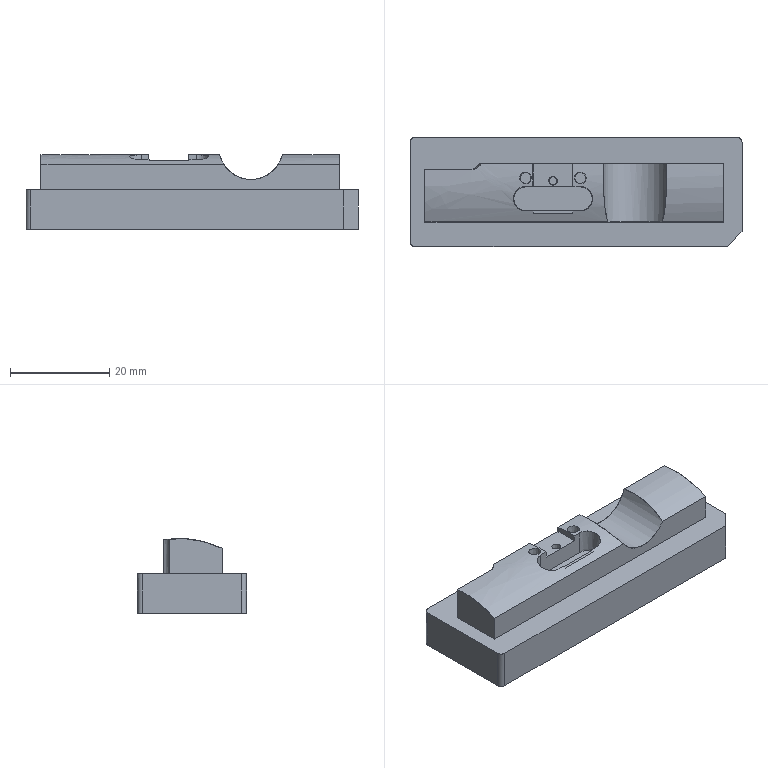NC program | PowerMill | posted with a generic post | part box 67 x 22 x 15.086 mm
Lines 1 to 1034 of 221347:
%
O0001
N104 ( POWERMILL CB  : 2026004.0)
N105 ( POST VER      : 2026.0.0.5161)
N106 ( OPTION FILE   : FANUC)
N107 ( OUTPUT WORKPLANE : WORLD)
N108 (  )
N109 ( TOOL LIST )
N110 (---------------------------------------)
N111 ( NO. | ID        | DIA.| TIP RAD|LENGTH)
N112 (---------------------------------------)
N113 (    1|D10C_1_1   |10.0 |  0.0   |70.52 )
N114 (   15|D3C_1_1    | 3.0 |  0.0   |62.28 )
N115 (   27|D1C_1_1    | 1.0 |  0.0   | 60.2 )
N116 (    3|D10_1_1    |10.0 |  0.0   |70.24 )
N117 (   22|R1.5_1_1   | 3.0 |  1.5   |60.28 )
N118 (   10|D3_1_1_1_1 | 3.0 |  0.0   |62.36 )
N119 (    8|D1_1_1     | 1.0 |  0.0   |60.28 )
N120 (   13|TEXT_D4_1_1| 4.0 |  0.3   |62.36 )
N121 (---------------------------------------)
N122 (  )
N123 ( NUMBER OF TOOLPATHS: 17.0 )
N124 ( ESTIMATED PROGRAM DURATION: 0 HOURS 24 MIN 1 SEC)
N125 (  )
N126 G00 G21 G80 G40 G17
N127 G90
N128 G54
N129 G53 Z0.0
N130 (---------------)
N131 ( START TOOLPATH : 精公开粗01-扫面平行-D10C )
N132 (---------------)
N133 ( TOOL NO.    :1 )
N134 ( TOOL TYPE   : ENDMILL)
N135 ( TOOL ID     : D10C_1_1)
N136 ( TOOL DIA    : 10.0 LENGTH 70.52)
N137 T1
N138 M6
N139 S8000 M03
N140 G00 G90 X0.0 Y0.0
N141 G43 Z10.2 H1
N142
N143 G05 P10000 R4
N144 X41.28 Y13.78
N145 Z1.125
N146 G01 Z-0.075 F6000.0
N147 X36.28 F10000.0
N148 X-36.28
N149 Y8.268
N150 X36.28
N151 Y2.756
N152 X-36.28
N153 Y-2.756
N154 X36.28
N155 Y-8.268
N156 X-36.28
N157 Y-13.78
N158 X36.28
N159 X41.28
N160 G00 Z10.2
N161 G05 P0
N162 (---------------)
N163 ( END TOOLPATH : 精公开粗01-扫面平行-D10C )
N164 (---------------)
N165 ( START TOOLPATH : 精公开粗01-外形偏置-D10C )
N166 (---------------)
N167 G00 X-0.3595 Y-0.0315 Z9.875
N168 G05 P10000 R4
N169 X42.812 Y10.5168
N170 Z0.7651
N171 G01 Z-0.4349 F6000.0
N172 X42.2845 F10000.0
N173 G03 X37.537 Y5.7693 I0.0 J-4.7475
N174 G01 Y-12.843
N175 G02 X36.537 Y-13.843 I-1.0 J0.0
N176 G01 X-4.6555
N177 Y-9.343
N178 Y-13.843
N179 X-37.256
N180 G02 X-38.256 Y-12.843 I0.0 J1.0
N181 G01 Y12.78
N182 G02 X-37.256 Y13.78 I1.0 J0.0
N183 G01 X36.537
N184 G02 X37.537 Y12.78 I0.0 J-1.0
N185 G01 Y5.7693
N186 X35.0391 Y5.7692
N187 X35.0394 Y-0.4182
N188 X35.0002 Y-1.1916
N189 X34.8777 Y-1.9651
N190 X34.646 Y-2.7385
N191 X34.4447 Y-3.2074
N192 X34.2765 Y-3.5119
N193 X33.7323 Y-4.2853
N194 X32.8978 Y-5.0686
N195 X32.1244 Y-5.5508
N196 X31.4565 Y-5.8322
N197 X31.4523 Y-5.8341
N198 X31.351 Y-5.879
N199 X30.5776 Y-6.0617
N200 X29.8041 Y-6.1276
N201 X29.0307 Y-6.0737
N202 X22.8433 Y-6.0671
N203 X18.2027 Y-6.1347
N204 X17.4293 Y-6.0783
N205 X16.6559 Y-5.9081
N206 X15.8825 Y-5.6028
N207 X15.109 Y-5.1333
N208 X14.3356 Y-4.4439
N209 X14.1974 Y-4.2853
N210 X13.6534 Y-3.5119
N211 X13.2864 Y-2.7385
N212 X13.056 Y-1.9651
N213 X12.9414 Y-1.1916
N214 X12.9113 Y-0.4182
N215 X12.9127 Y5.7692
N216 Y5.7697
N217 X10.8981 Y5.7692
N218 X10.8998 Y-0.4182
N219 X10.8699 Y-1.1916
N220 X10.7526 Y-1.9651
N221 X10.5252 Y-2.7385
N222 X10.1573 Y-3.5119
N223 X9.695 Y-4.1892
N224 X8.9216 Y-4.961
N225 X8.1482 Y-5.4778
N226 X7.3727 Y-5.8322
N227 X6.6013 Y-6.0395
N228 X5.8279 Y-6.1271
N229 X4.2811 Y-6.1333
N230 X2.7342 Y-6.0999
N231 X1.9608 Y-5.9598
N232 X1.5441 Y-5.8322
N233 X1.1874 Y-5.6899
N234 X0.4139 Y-5.2772
N235 X-0.3595 Y-4.6536
N236 X-0.6368 Y-4.3496
N237 G03 X-0.9766 Y-4.1874 I-0.3694 J-0.3369
N238 G01 X-1.1329 Y-4.1781
N239 X-1.9064 Y-4.0467
N240 X-2.6798 Y-3.7923
N241 X-3.2518 Y-3.5119
N242 X-3.4532 Y-3.3884
N243 X-4.2266 Y-2.796
N244 X-4.2994 Y-2.7209
N245 G03 X-5.021 Y-2.7244 I-0.3591 J-0.3479
N246 G01 X-5.0344 Y-2.7385
N247 X-5.7735 Y-3.325
N248 X-6.075 Y-3.5119
N249 X-6.5469 Y-3.7506
N250 X-7.3203 Y-4.0226
N251 X-8.0938 Y-4.1681
N252 X-8.3143 Y-4.1838
N253 G03 X-8.6511 Y-4.3489 I0.0356 J-0.4988
N254 G01 X-8.8672 Y-4.5901
N255 X-9.6406 Y-5.2349
N256 X-10.414 Y-5.6575
N257 X-10.8395 Y-5.8322
N258 X-11.1875 Y-5.9403
N259 X-11.9609 Y-6.095
N260 X-12.7343 Y-6.1333
N261 X-29.7497 Y-6.0944
N262 X-30.5231 Y-6.1271
N263 X-31.2966 Y-6.0617
N264 X-32.07 Y-5.8777
N265 X-32.8434 Y-5.5543
N266 X-33.6168 Y-5.0722
N267 X-34.3903 Y-4.3585
N268 X-34.9974 Y-3.5119
N269 X-35.1637 Y-3.1988
N270 X-35.3656 Y-2.7385
N271 X-35.5964 Y-1.9651
N272 X-35.7176 Y-1.1916
N273 X-35.7567 Y-0.4182
N274 Y4.2223
N275 X-35.7341 Y4.9958
N276 X-35.6038 Y5.7692
N277 X-35.3487 Y6.5426
N278 X-35.1637 Y6.9387
N279 X-34.9478 Y7.3161
N280 X-34.3903 Y8.0519
N281 X-33.6168 Y8.7523
N282 X-32.8434 Y9.2273
N283 X-32.07 Y9.5414
N284 X-31.2966 Y9.7235
N285 X-30.5231 Y9.7872
N286 X-22.6611 Y9.7875
N287 X-22.5083 Y9.8115
N288 X-22.3701 Y9.8809
N289 X-22.0154 Y10.1347
N290 X-21.543 Y10.4098
N291 X-21.242 Y10.5544
N292 X-20.4686 Y10.8156
N293 X-19.6952 Y10.9584
N294 X-18.9217 Y10.9875
N295 X-8.8672
N296 X-8.0938 Y10.9541
N297 X-7.3203 Y10.8087
N298 X-6.5469 Y10.5359
N299 X-6.2787 Y10.4098
N300 X-5.7735 Y10.1145
N301 X-5.1563 Y9.6363
N302 X-5.0205 Y9.4979
N303 G03 X-4.3059 Y9.499 I0.3568 J0.3503
N304 G01 X-4.1718 Y9.6363
N305 X-3.4532 Y10.1782
N306 X-3.0458 Y10.4098
N307 X-2.6798 Y10.5795
N308 X-1.9064 Y10.8344
N309 X-1.1329 Y10.9648
N310 X-0.3595 Y10.9875
N311 X5.8279 Y10.9778
N312 X6.6013 Y10.8926
N313 X7.3748 Y10.6845
N314 X8.0172 Y10.4098
N315 X8.9216 Y9.8251
N316 X9.1445 Y9.6363
N317 X9.695 Y9.0614
N318 X9.851 Y8.8629
N319 X10.3302 Y8.0895
N320 X10.4685 Y7.7926
N321 X10.6473 Y7.3161
N322 X10.8319 Y6.5426
N323 X10.8981 Y5.7692
N324 X12.9127 Y5.7697
N325 X12.9788 Y6.5426
N326 X13.1635 Y7.3161
N327 X13.4806 Y8.0895
N328 X13.9597 Y8.8629
N329 X14.3356 Y9.3119
N330 X14.6663 Y9.6363
N331 X15.109 Y9.9921
N332 X15.7931 Y10.4098
N333 X16.6559 Y10.758
N334 X17.4293 Y10.9307
N335 X18.2027 Y10.9875
N336 X29.8041 Y10.9873
N337 X30.5776 Y10.9237
N338 X31.351 Y10.742
N339 X32.1244 Y10.4282
N340 X32.8978 Y9.9536
N341 X33.2869 Y9.6363
N342 X33.6713 Y9.2538
N343 X33.9929 Y8.8629
N344 X34.4447 Y8.1421
N345 X34.7885 Y7.3161
N346 X34.973 Y6.5426
N347 X35.0391 Y5.7692
N348 X37.537 Y5.7693
N349 G00 Z3.4552
N350 G01 X42.812 Y10.5168
N351 G00 Z0.4552
N352 G01 Z-0.7448 F6000.0
N353 X42.2845 F10000.0
N354 G03 X37.537 Y5.7693 I0.0 J-4.7475
N355 G01 X35.0391 Y5.7692
N356 X35.0394 Y-1.9651
N357 X34.9965 Y-2.7385
N358 X34.8575 Y-3.5119
N359 X34.5995 Y-4.2853
N360 X34.4447 Y-4.6234
N361 X34.1992 Y-5.0588
N362 X33.6713 Y-5.7649
N363 X32.8978 Y-6.4773
N364 X32.1244 Y-6.9589
N365 X31.351 Y-7.2764
N366 X30.9778 Y-7.3791
N367 X30.5776 Y-7.4603
N368 X29.8041 Y-7.5246
N369 X29.0307 Y-7.4886
N370 X22.0699 Y-7.4915
N371 X22.0674
N372 X18.2027 Y-7.5315
N373 X17.4293 Y-7.4943
N374 X16.8293 Y-7.3791
N375 X15.8825 Y-7.047
N376 X15.109 Y-6.6057
N377 X14.3356 Y-5.9511
N378 X14.2228 Y-5.8322
N379 X13.6358 Y-5.0588
N380 X13.24 Y-4.2853
N381 X12.9867 Y-3.5119
N382 X12.854 Y-2.7385
N383 X12.8131 Y-1.9651
N384 X12.8076 Y-1.1916
N385 X12.8105 Y4.9958
N386 X12.8069 Y5.7677
N387 X11.0044 Y5.7692
N388 X10.9979 Y-1.9651
N389 X10.9566 Y-2.7385
N390 X10.824 Y-3.5119
N391 X10.5684 Y-4.2853
N392 X10.4685 Y-4.515
N393 X10.1725 Y-5.0588
N394 X9.695 Y-5.7093
N395 X8.9216 Y-6.4452
N396 X8.1482 Y-6.9381
N397 X7.3748 Y-7.2651
N398 X6.9832 Y-7.3791
N399 X6.6013 Y-7.4577
N400 X5.8279 Y-7.5317
N401 X2.7342 Y-7.5219
N402 X1.9608 Y-7.4019
N403 X1.1874 Y-7.1556
N404 X0.4139 Y-6.7672
N405 X0.1665 Y-6.6056
N406 X-0.3595 Y-6.1917
N407 X-0.7158 Y-5.8322
N408 X-1.1329 Y-5.319
N409 X-1.306 Y-5.0588
N410 X-1.6968 Y-4.2853
N411 X-1.7914 Y-4.142
N412 X-1.929 Y-4.0392
N413 X-2.4752 Y-3.8595
N414 X-2.6798 Y-3.7948
N415 X-2.7651 Y-3.7504
N416 X-3.2518 Y-3.5119
N417 X-3.412 Y-3.4136
N418 X-3.4532 Y-3.3922
N419 X-4.2266 Y-2.7991
N420 X-4.2965 Y-2.7267
N421 G03 X-5.0202 Y-2.731 I-0.3598 J-0.3472
N422 G01 X-5.0272 Y-2.7385
N423 X-5.7735 Y-3.3321
N424 X-6.0667 Y-3.5119
N425 X-6.5469 Y-3.7538
N426 X-7.2969 Y-4.0174
N427 G03 X-7.5877 Y-4.2853 I0.1658 J-0.4717
N428 G01 X-7.9842 Y-5.0588
N429 X-8.5712 Y-5.8322
N430 X-8.8672 Y-6.1355
N431 X-9.6406 Y-6.7332
N432 X-10.414 Y-7.1284
N433 X-11.1875 Y-7.3812
N434 X-11.9609 Y-7.5166
N435 X-12.7343 Y-7.532
N436 X-20.4686 Y-7.5073
N437 X-29.7497 Y-7.4879
N438 X-30.5231 Y-7.5246
N439 X-31.2966 Y-7.46
N440 X-32.07 Y-7.2758
N441 X-32.8434 Y-6.958
N442 X-33.6168 Y-6.476
N443 X-34.3272 Y-5.8322
N444 X-34.9166 Y-5.0588
N445 X-35.1637 Y-4.62
N446 X-35.3166 Y-4.2853
N447 X-35.5746 Y-3.5119
N448 X-35.7145 Y-2.7385
N449 X-35.7567 Y-1.9651
N450 Y4.2223
N451 X-35.7341 Y4.9958
N452 X-35.6038 Y5.7692
N453 X-35.3487 Y6.5426
N454 X-35.1637 Y6.9387
N455 X-34.9478 Y7.3161
N456 X-34.3903 Y8.0519
N457 X-33.6168 Y8.7523
N458 X-32.8434 Y9.2273
N459 X-32.07 Y9.5414
N460 X-31.2966 Y9.7235
N461 X-30.5231 Y9.7872
N462 X-22.6793 Y9.7875
N463 X-22.5248 Y9.812
N464 X-22.3854 Y9.883
N465 X-22.0154 Y10.1519
N466 X-21.5666 Y10.4098
N467 X-21.242 Y10.5619
N468 X-20.4686 Y10.8215
N469 X-19.6952 Y10.9608
N470 X-18.9217 Y10.9875
N471 X-8.8672
N472 X-8.0938 Y10.9547
N473 X-7.3203 Y10.8093
N474 X-6.5469 Y10.537
N475 X-6.2775 Y10.4098
N476 X-5.7735 Y10.1157
N477 X-5.1516 Y9.6363
N478 X-5.0198 Y9.5012
N479 G03 X-4.304 Y9.5009 I0.358 J0.349
N480 G01 X-4.1718 Y9.6363
N481 X-3.4532 Y10.1784
N482 X-3.0459 Y10.4098
N483 X-2.6798 Y10.5797
N484 X-1.9064 Y10.8348
N485 X-1.1329 Y10.9649
N486 X-0.3595 Y10.9875
N487 X5.8279 Y10.9859
N488 X6.6013 Y10.9124
N489 X7.3748 Y10.7207
N490 X8.1234 Y10.4098
N491 X8.9216 Y9.9077
N492 X9.2502 Y9.6363
N493 X9.695 Y9.1855
N494 X9.9568 Y8.8629
N495 X10.436 Y8.0895
N496 X10.753 Y7.3161
N497 X10.9377 Y6.5426
N498 X11.0044 Y5.7692
N499 X12.8069 Y5.7677
N500 Y5.7692
N501 X12.873 Y6.5426
N502 X13.0577 Y7.3161
N503 X13.3748 Y8.0895
N504 X13.5622 Y8.4268
N505 X13.8539 Y8.8629
N506 X14.3356 Y9.4218
N507 X14.5605 Y9.6363
N508 X15.109 Y10.0662
N509 X15.8825 Y10.5029
N510 X16.6559 Y10.7877
N511 X17.4293 Y10.9459
N512 X18.2027 Y10.9875
N513 X29.8041 Y10.9874
N514 X30.5776 Y10.9237
N515 X31.351 Y10.742
N516 X32.1244 Y10.4282
N517 X32.8978 Y9.9536
N518 X33.2869 Y9.6363
N519 X33.6713 Y9.2538
N520 X33.993 Y8.8629
N521 X34.4447 Y8.1421
N522 X34.7885 Y7.3161
N523 X34.973 Y6.5426
N524 X35.0391 Y5.7692
N525 X37.537 Y5.7693
N526 Y-12.843
N527 G02 X36.537 Y-13.843 I-1.0 J0.0
N528 G01 X-37.256
N529 G02 X-38.256 Y-12.843 I0.0 J1.0
N530 G01 Y12.78
N531 G02 X-37.256 Y13.78 I1.0 J0.0
N532 G01 X36.537
N533 G02 X37.537 Y12.78 I0.0 J-1.0
N534 G01 Y5.7693
N535 G00 Z3.1453
N536 G01 X42.812 Y10.5168
N537 G00 Z0.1453
N538 G01 Z-1.0547 F6000.0
N539 X42.2845 F10000.0
N540 G03 X37.537 Y5.7693 I0.0 J-4.7475
N541 G01 Y-12.843
N542 G02 X36.537 Y-13.843 I-1.0 J0.0
N543 G01 X-37.256
N544 G02 X-38.256 Y-12.843 I0.0 J1.0
N545 G01 Y12.78
N546 G02 X-37.256 Y13.78 I1.0 J0.0
N547 G01 X36.537
N548 G02 X37.537 Y12.78 I0.0 J-1.0
N549 G01 Y5.7693
N550 X35.0391 Y5.7692
N551 X35.0395 Y-2.7385
N552 X35.0271 Y-3.5119
N553 X34.927 Y-4.2853
N554 X34.7154 Y-5.0588
N555 X34.4447 Y-5.6949
N556 X33.8643 Y-6.6056
N557 X33.6713 Y-6.8349
N558 X33.1133 Y-7.3791
N559 X32.8978 Y-7.5485
N560 X32.1244 Y-8.0291
N561 X31.861 Y-8.1525
N562 X31.351 Y-8.3489
N563 X30.5776 Y-8.533
N564 X29.8041 Y-8.5973
N565 X18.2027 Y-8.5978
N566 X17.4293 Y-8.5703
N567 X16.6559 Y-8.4306
N568 X15.8538 Y-8.1525
N569 X15.109 Y-7.7483
N570 X14.6116 Y-7.3791
N571 X14.3356 Y-7.1327
N572 X13.8585 Y-6.6056
N573 X13.5622 Y-6.1899
N574 X13.3534 Y-5.8322
N575 X13.0146 Y-5.0588
N576 X12.8064 Y-4.2853
N577 X12.7134 Y-3.5119
N578 X12.7053 Y-2.7385
N579 X12.7067 Y4.9958
N580 X12.7066 Y4.9976
N581 X12.7011 Y5.7639
N582 X11.1106 Y5.7692
N583 X11.1055 Y4.2223
N584 X11.1057 Y-2.7385
N585 X11.0978 Y-3.5119
N586 X11.004 Y-4.2853
N587 X10.7982 Y-5.0588
N588 X10.4685 Y-5.817
N589 X9.9511 Y-6.6056
N590 X9.695 Y-6.9088
N591 X9.1998 Y-7.3791
N592 X8.9216 Y-7.5981
N593 X8.1482 Y-8.0644
N594 X7.9522 Y-8.1525
N595 X7.3748 Y-8.3693
N596 X6.6013 Y-8.5439
N597 X5.8279 Y-8.5965
N598 X1.9608 Y-8.5906
N599 X1.1874 Y-8.4834
N600 X0.4139 Y-8.2572
N601 X-0.3595 Y-7.8923
N602 X-1.0844 Y-7.3791
N603 X-1.8243 Y-6.6056
N604 X-2.34 Y-5.8322
N605 X-2.6798 Y-5.0118
N606 X-2.8627 Y-4.2853
N607 X-2.9017 Y-3.9413
N608 G03 X-3.1559 Y-3.5604 I-0.4968 J-0.0563
N609 G01 X-3.1803 Y-3.5469
N610 X-3.2518 Y-3.5118
N611 X-3.3308 Y-3.4634
N612 X-3.4532 Y-3.3954
N613 X-4.2266 Y-2.8021
N614 X-4.2943 Y-2.7318
N615 G03 X-5.0199 Y-2.7369 I-0.3603 J-0.3466
N616 G01 X-5.0214 Y-2.7385
N617 X-5.7735 Y-3.3356
N618 X-5.8594 Y-3.3847
N619 X-6.0667 Y-3.5119
N620 X-6.1637 Y-3.5607
N621 G03 X-6.3775 Y-3.9194 I0.2833 J-0.412
N622 G01 X-6.4168 Y-4.2853
N623 X-6.6201 Y-5.0588
N624 X-6.9545 Y-5.8322
N625 X-7.4607 Y-6.6056
N626 X-8.0938 Y-7.2856
N627 X-8.8672 Y-7.8515
N628 X-9.6406 Y-8.2314
N629 X-10.414 Y-8.4724
N630 X-11.1875 Y-8.5863
N631 X-30.5231 Y-8.5972
N632 X-31.2966 Y-8.5328
N633 X-32.07 Y-8.3483
N634 X-32.5855 Y-8.1525
N635 X-32.8434 Y-8.0285
N636 X-33.6168 Y-7.5477
N637 X-33.8307 Y-7.3791
N638 X-34.3903 Y-6.8332
N639 X-34.5817 Y-6.6056
N640 X-35.0898 Y-5.8322
N641 X-35.4338 Y-5.0588
N642 X-35.6443 Y-4.2853
N643 X-35.7407 Y-3.5119
N644 X-35.7567 Y-2.7385
N645 Y4.2223
N646 X-35.7341 Y4.9958
N647 X-35.6038 Y5.7692
N648 X-35.3487 Y6.5426
N649 X-35.1637 Y6.9387
N650 X-34.9478 Y7.3161
N651 X-34.3903 Y8.0519
N652 X-33.6168 Y8.7523
N653 X-32.8434 Y9.2274
N654 X-32.07 Y9.5414
N655 X-31.2966 Y9.7235
N656 X-30.5231 Y9.7872
N657 X-22.6951 Y9.7875
N658 X-22.5411 Y9.8118
N659 X-22.4021 Y9.8824
N660 X-22.0154 Y10.162
N661 X-21.583 Y10.4098
N662 X-21.242 Y10.5685
N663 X-20.4686 Y10.8275
N664 X-19.6952 Y10.9625
N665 X-18.9217 Y10.9875
N666 X-8.8672
N667 X-8.0938 Y10.9552
N668 X-7.3203 Y10.8099
N669 X-6.5469 Y10.5382
N670 X-6.2763 Y10.4098
N671 X-5.7735 Y10.117
N672 X-5.1504 Y9.6363
N673 X-5.0192 Y9.5018
N674 G03 X-4.3033 Y9.5016 I0.358 J0.349
N675 G01 X-4.1719 Y9.6363
N676 X-3.4532 Y10.1786
N677 X-3.0459 Y10.4098
N678 X-2.6798 Y10.5799
N679 X-1.9064 Y10.8351
N680 X-1.1329 Y10.9649
N681 X-0.3595 Y10.9875
N682 X5.8279
N683 X6.6013 Y10.93
N684 X7.3748 Y10.7552
N685 X8.1482 Y10.4513
N686 X8.9216 Y9.9863
N687 X9.356 Y9.6363
N688 X9.695 Y9.303
N689 X10.0626 Y8.8629
N690 X10.4685 Y8.2294
N691 X10.8588 Y7.3161
N692 X11.0435 Y6.5426
N693 X11.1106 Y5.7692
N694 X12.7011 Y5.7639
N695 Y5.7692
N696 X12.7672 Y6.5426
N697 X12.9519 Y7.3161
N698 X13.269 Y8.0895
N699 X13.5622 Y8.5981
N700 X13.7481 Y8.8629
N701 X14.3356 Y9.5263
N702 X15.109 Y10.1368
N703 X15.5815 Y10.4098
N704 X15.8825 Y10.5517
N705 X16.6559 Y10.8174
N706 X17.4293 Y10.9579
N707 X18.2027 Y10.9875
N708 X29.8041 Y10.9874
N709 X30.5776 Y10.9237
N710 X31.351 Y10.742
N711 X32.1244 Y10.4282
N712 X32.8978 Y9.9536
N713 X33.2869 Y9.6363
N714 X33.6713 Y9.2539
N715 X33.993 Y8.8629
N716 X34.4447 Y8.1422
N717 X34.7885 Y7.3161
N718 X34.973 Y6.5426
N719 X35.0391 Y5.7692
N720 X37.537 Y5.7693
N721 G00 Z2.8354
N722 G01 X42.812 Y10.5168
N723 G00 Z-0.1646
N724 G01 Z-1.3646 F6000.0
N725 X42.2845 F10000.0
N726 G03 X37.537 Y5.7693 I0.0 J-4.7475
N727 G01 X35.0391 Y5.7692
N728 X35.0393 Y1.0471
N729 X35.0394 Y-2.7385
N730 Y-2.7412
N731 Y-3.5119
N732 X35.0333 Y-4.2853
N733 X34.9464 Y-5.0588
N734 X34.7498 Y-5.8322
N735 X34.4447 Y-6.5662
N736 X33.9363 Y-7.3791
N737 X33.6713 Y-7.701
N738 X33.2184 Y-8.1525
N739 X32.8978 Y-8.4127
N740 X32.0534 Y-8.9259
N741 X31.351 Y-9.2122
N742 X30.5776 Y-9.3959
N743 X29.8041 Y-9.4601
N744 X18.2027 Y-9.4822
N745 X17.4293 Y-9.4648
N746 X16.6559 Y-9.3468
N747 X15.8825 Y-9.1037
N748 X15.4867 Y-8.9259
N749 X15.109 Y-8.7179
N750 X14.3475 Y-8.1525
N751 X13.6396 Y-7.3791
N752 X13.1581 Y-6.6056
N753 X12.8404 Y-5.8322
N754 X12.6496 Y-5.0588
N755 X12.5659 Y-4.2853
N756 X12.5662 Y5.7692
N757 X12.5751 Y5.8735
N758 X11.2419
N759 Y-4.3477
N760 X11.1606 Y-5.0588
N761 X10.9694 Y-5.8322
N762 X10.651 Y-6.6056
N763 X10.4685 Y-6.9369
N764 X10.1701 Y-7.3791
N765 X9.695 Y-7.9313
N766 X9.4592 Y-8.1525
N767 X8.9216 Y-8.5741
N768 X8.317 Y-8.9259
N769 X8.1482 Y-9.0094
N770 X7.3748 Y-9.2891
N771 X6.6013 Y-9.4431
N772 X5.8279 Y-9.4796
N773 X0.4139 Y-9.4801
N774 X-1.1329 Y-9.4604
N775 X-1.9064 Y-9.3245
N776 X-2.6798 Y-9.0659
N777 X-2.9783 Y-8.9259
N778 X-3.4532 Y-8.6592
N779 X-4.1204 Y-8.1525
N780 X-4.2994 Y-7.9688
N781 G03 X-5.016 Y-7.969 I-0.3582 J-0.3488
N782 G01 X-5.1944 Y-8.1525
N783 X-5.7735 Y-8.6005
N784 X-6.5469 Y-9.0268
N785 X-7.3203 Y-9.3012
N786 X-8.0938 Y-9.4475
N787 X-8.8672 Y-9.4801
N788 X-30.5231 Y-9.4752
N789 X-31.2966 Y-9.4102
N790 X-32.07 Y-9.2263
N791 X-32.8434 Y-8.9083
N792 X-33.6168 Y-8.4271
N793 X-33.9527 Y-8.1525
N794 X-34.3903 Y-7.7145
N795 X-34.6635 Y-7.3791
N796 X-35.1637 Y-6.5765
N797 X-35.4708 Y-5.8322
N798 X-35.6657 Y-5.0588
N799 X-35.75 Y-4.2853
N800 X-35.7567 Y-3.5119
N801 Y4.2223
N802 X-35.7341 Y4.9958
N803 X-35.6038 Y5.7692
N804 X-35.3487 Y6.5426
N805 X-35.1637 Y6.9387
N806 X-34.9478 Y7.3161
N807 X-34.3903 Y8.0519
N808 X-33.6168 Y8.7523
N809 X-32.8434 Y9.2274
N810 X-32.07 Y9.5414
N811 X-31.2966 Y9.7235
N812 X-30.5231 Y9.7872
N813 X-22.7109 Y9.7875
N814 X-22.5574 Y9.8117
N815 X-22.4188 Y9.8818
N816 X-22.0154 Y10.1721
N817 X-21.5993 Y10.4098
N818 X-21.242 Y10.575
N819 X-20.4686 Y10.8323
N820 X-19.6952 Y10.9641
N821 X-18.9217 Y10.9875
N822 X-8.8672
N823 X-8.0938 Y10.9561
N824 X-7.3203 Y10.8116
N825 X-6.5469 Y10.5412
N826 X-6.503 Y10.5173
N827 X-6.2763 Y10.4097
N828 X-5.8426 Y10.1571
N829 X-5.7735 Y10.1195
N830 X-5.1492 Y9.6363
N831 X-5.0186 Y9.5024
N832 G03 X-4.3028 Y9.5022 I0.358 J0.3491
N833 G01 X-4.1719 Y9.6363
N834 X-3.4532 Y10.1787
N835 X-3.0459 Y10.4098
N836 X-2.6798 Y10.5801
N837 X-1.9064 Y10.8354
N838 X-1.1329 Y10.965
N839 X-0.3595 Y10.9875
N840 X5.8279
N841 X6.6013 Y10.9476
N842 X7.3748 Y10.7938
N843 X8.1482 Y10.5129
N844 X8.9216 Y10.0792
N845 X9.4901 Y9.6363
N846 X9.695 Y9.4426
N847 X10.1973 Y8.8629
N848 X10.4685 Y8.462
N849 X10.6769 Y8.0895
N850 X10.9939 Y7.3161
N851 X11.1793 Y6.5426
N852 X11.2419 Y5.8735
N853 X12.5751
N854 X12.6323 Y6.5426
N855 X12.7888 Y7.223
N856 X13.1343 Y8.0895
N857 X13.5622 Y8.7918
N858 X14.321 Y9.6363
N859 X15.109 Y10.2211
N860 X15.4491 Y10.4098
N861 X15.8825 Y10.6071
N862 X16.6559 Y10.8505
N863 X17.4293 Y10.9698
N864 X18.2027 Y10.9876
N865 X29.8041 Y10.9874
N866 X30.5776 Y10.9237
N867 X31.351 Y10.742
N868 X32.1244 Y10.4282
N869 X32.8978 Y9.9536
N870 X33.2869 Y9.6363
N871 X33.6713 Y9.2539
N872 X33.993 Y8.8629
N873 X34.4447 Y8.1422
N874 X34.7885 Y7.3161
N875 X34.973 Y6.5426
N876 X35.0391 Y5.7692
N877 X37.537 Y5.7693
N878 Y-12.843
N879 G02 X36.537 Y-13.843 I-1.0 J0.0
N880 G01 X-37.256
N881 G02 X-38.256 Y-12.843 I0.0 J1.0
N882 G01 Y12.78
N883 G02 X-37.256 Y13.78 I1.0 J0.0
N884 G01 X36.537
N885 G02 X37.537 Y12.78 I0.0 J-1.0
N886 G01 Y5.7693
N887 G00 Z2.453
N888 G01 X42.812 Y10.5168
N889 G00 Z-0.547
N890 G01 Z-1.747 F6000.0
N891 X42.2845 F10000.0
N892 G03 X37.537 Y5.7693 I0.0 J-4.7475
N893 G01 X35.0391 Y5.7692
N894 X35.0393 Y-0.9925
N895 X35.0394 Y-2.7385
N896 Y-2.7402
N897 Y-5.0588
N898 X34.9829 Y-5.8322
N899 X34.8192 Y-6.6056
N900 X34.5304 Y-7.3791
N901 X34.0937 Y-8.1525
N902 X33.6713 Y-8.6955
N903 X33.4521 Y-8.9259
N904 X32.8978 Y-9.4057
N905 X32.4577 Y-9.6993
N906 X32.1244 Y-9.886
N907 X31.351 Y-10.2032
N908 X30.5776 Y-10.3869
N909 X29.8041 Y-10.4508
N910 X18.2027 Y-10.4511
N911 X17.4293 Y-10.4449
N912 X16.6559 Y-10.3576
N913 X15.8825 Y-10.1478
N914 X15.109 Y-9.8003
N915 X14.3356 Y-9.2772
N916 X13.9485 Y-8.9259
N917 X13.5622 Y-8.4997
N918 X13.3071 Y-8.1525
N919 X12.8718 Y-7.3791
N920 X12.5896 Y-6.6056
N921 X12.4315 Y-5.8322
N922 X12.3851 Y-5.0588
N923 X12.3848 Y4.9958
N924 X12.3847 Y4.9986
N925 X12.3762 Y5.7591
N926 X11.434 Y5.7692
N927 X11.4257 Y4.9958
N928 X11.4262 Y-5.0588
N929 X11.378 Y-5.8322
N930 X11.2419 Y-6.5326
N931 X10.9371 Y-7.3791
N932 X10.5031 Y-8.1525
N933 X9.862 Y-8.9259
N934 X9.695 Y-9.0878
N935 X8.8701 Y-9.6993
N936 X8.1482 Y-10.064
N937 X7.3748 Y-10.3105
N938 X6.6013 Y-10.4314
N939 X5.8279 Y-10.4509
N940 X-30.5231 Y-10.451
N941 X-31.2966 Y-10.3864
N942 X-32.07 Y-10.2027
N943 X-32.8434 Y-9.885
N944 X-33.1739 Y-9.6993
N945 X-33.6168 Y-9.4044
N946 X-34.1675 Y-8.9259
N947 X-34.3903 Y-8.6936
N948 X-34.8121 Y-8.1525
N949 X-35.1637 Y-7.5576
N950 X-35.5359 Y-6.6056
N951 X-35.7005 Y-5.8322
N952 X-35.7567 Y-5.0588
N953 Y4.2223
N954 X-35.7341 Y4.9958
N955 X-35.6038 Y5.7692
N956 X-35.3487 Y6.5426
N957 X-35.1637 Y6.9387
N958 X-34.9478 Y7.3161
N959 X-34.3903 Y8.0519
N960 X-33.6168 Y8.7523
N961 X-32.8434 Y9.2274
N962 X-32.07 Y9.5414
N963 X-31.2966 Y9.7235
N964 X-30.5231 Y9.7872
N965 X-22.73 Y9.7875
N966 X-22.577 Y9.8115
N967 X-22.4387 Y9.8811
N968 X-22.0154 Y10.1845
N969 X-21.6194 Y10.4098
N970 X-21.242 Y10.5832
N971 X-20.4686 Y10.8372
N972 X-19.6952 Y10.9659
N973 X-18.9217 Y10.9875
N974 X5.8279
N975 X6.6013 Y10.9671
N976 X7.3748 Y10.8422
N977 X8.1482 Y10.5935
N978 X8.551 Y10.4098
N979 X8.9216 Y10.2021
N980 X9.695 Y9.6223
N981 X10.3869 Y8.8629
N982 X10.8655 Y8.0895
N983 X11.1837 Y7.3161
N984 X11.3677 Y6.5426
N985 X11.434 Y5.7692
N986 X12.3762 Y5.7591
N987 X12.3761 Y5.7692
N988 X12.4431 Y6.5426
N989 X12.6279 Y7.3161
N990 X12.7888 Y7.7509
N991 X12.9453 Y8.0895
N992 X13.4247 Y8.8629
N993 X13.5622 Y9.038
N994 X14.1319 Y9.6363
N995 X14.3356 Y9.8095
N996 X15.109 Y10.3297
N997 X15.8825 Y10.6788
N998 X16.6559 Y10.89
N999 X17.4293 Y10.9818
N1000 X18.2027 Y10.9876
N1001 X29.8041 Y10.9874
N1002 X30.5776 Y10.9237
N1003 X31.351 Y10.742
N1004 X32.1244 Y10.4282
N1005 X32.8978 Y9.9536
N1006 X33.2869 Y9.6363
N1007 X33.6713 Y9.2539
N1008 X33.993 Y8.8629
N1009 X34.4447 Y8.1422
N1010 X34.7885 Y7.3161
N1011 X34.973 Y6.5426
N1012 X35.0391 Y5.7692
N1013 X37.537 Y5.7693
N1014 Y-12.843
N1015 G02 X36.537 Y-13.843 I-1.0 J0.0
N1016 G01 X-37.256
N1017 G02 X-38.256 Y-12.843 I0.0 J1.0
N1018 G01 Y12.78
N1019 G02 X-37.256 Y13.78 I1.0 J0.0
N1020 G01 X36.537
N1021 G02 X37.537 Y12.78 I0.0 J-1.0
N1022 G01 Y5.7693
N1023 G00 Z2.0707
N1024 G01 X42.812 Y10.5168
N1025 G00 Z-0.9293
N1026 G01 Z-2.1293 F6000.0
N1027 X42.2845 F10000.0
N1028 G03 X37.537 Y5.7693 I0.0 J-4.7475
N1029 G01 Y-12.843
N1030 G02 X36.537 Y-13.843 I-1.0 J0.0
N1031 G01 X23.6168
N1032 X23.6167 Y-11.3387
N1033 X17.4293 Y-11.3389
N1034 X16.462 Y-11.2462
N1035 X15.8825 Y-11.0938
N1036 X15.109 Y-10.7899
N1037 X14.3356 Y-10.3269
N1038 X13.6227 Y-9.6993
N1039 X13.0098 Y-8.9259
N1040 X12.7888 Y-8.5504
N1041 X12.5969 Y-8.1525
N1042 X12.3318 Y-7.3791
N1043 X12.1926 Y-6.6056
N1044 X12.153 Y-5.8322
N1045 X12.1527 Y5.7692
N1046 X11.6581
N1047 X11.6571 Y-5.8322
N1048 X11.6174 Y-6.6056
N1049 X11.4794 Y-7.3791
N1050 X11.2419 Y-8.088
N1051 X10.8011 Y-8.9259
N1052 X10.4685 Y-9.3814
N1053 X10.1907 Y-9.6993
N1054 X9.695 Y-10.154
N1055 X9.2596 Y-10.4728
N1056 X8.9216 Y-10.6782
N1057 X8.1482 Y-11.0231
N1058 X7.3449 Y-11.2462
N1059 X6.6013 Y-11.325
N1060 X5.8279 Y-11.3389
N1061 X-30.5231 Y-11.3385
N1062 X-31.2966 Y-11.2731
N1063 X-32.07 Y-11.0925
N1064 X-32.8434 Y-10.7784
N1065 X-33.3731 Y-10.4728
N1066 X-33.6168 Y-10.3027
N1067 X-34.2965 Y-9.6993
N1068 X-34.908 Y-8.9259
N1069 X-35.1637 Y-8.4803
N1070 X-35.3204 Y-8.1525
N1071 X-35.5853 Y-7.3791
N1072 X-35.7233 Y-6.6056
N1073 X-35.7567 Y-5.8322
N1074 Y4.2223
N1075 X-35.7341 Y4.9958
N1076 X-35.6038 Y5.7692
N1077 X-35.3487 Y6.5426
N1078 X-35.1637 Y6.9388
N1079 X-34.9478 Y7.3161
N1080 X-34.3903 Y8.0519
N1081 X-33.6168 Y8.7523
N1082 X-32.8434 Y9.2274
N1083 X-32.07 Y9.5414
N1084 X-31.2966 Y9.7235
N1085 X-30.5231 Y9.7872
N1086 X-22.7498 Y9.7875
N1087 X-22.5974 Y9.8113
N1088 X-22.4596 Y9.8804
N1089 X-22.0154 Y10.197
N1090 X-21.6395 Y10.4098
N1091 X-21.242 Y10.5913
N1092 X-20.4686 Y10.8421
N1093 X-19.6952 Y10.9677
N1094 X-18.9217 Y10.9875
N1095 X5.8279
N1096 X6.6013 Y10.9821
N1097 X7.3748 Y10.8902
N1098 X8.1482 Y10.679
N1099 X8.7716 Y10.4098
N1100 X9.695 Y9.8106
N1101 X9.9013 Y9.6363
N1102 X10.4685 Y9.0416
N1103 X10.6104 Y8.8629
N1104 X11.0899 Y8.0895
N1105 X11.4067 Y7.3161
N1106 X11.5917 Y6.5426
N1107 X11.6581 Y5.7692
N1108 X12.1527
N1109 X12.2175 Y6.5426
N1110 X12.4036 Y7.3161
N1111 X12.7217 Y8.0895
N1112 X13.2017 Y8.8629
N1113 X13.5622 Y9.2941
N1114 X13.9097 Y9.6363
N1115 X14.3356 Y9.9792
N1116 X15.0392 Y10.4098
N1117 X15.8825 Y10.751
N1118 X16.6559 Y10.9276
N1119 X17.4293 Y10.9875
N1120 X18.1977
N1121 X18.2027
N1122 X22.8046 Y10.9874
N1123 X29.8041
N1124 X30.5776 Y10.9237
N1125 X31.351 Y10.742
N1126 X32.1244 Y10.4282
N1127 X32.8978 Y9.9536
N1128 X33.2869 Y9.6363
N1129 X33.6713 Y9.2539
N1130 X33.993 Y8.8629
N1131 X34.4447 Y8.1422